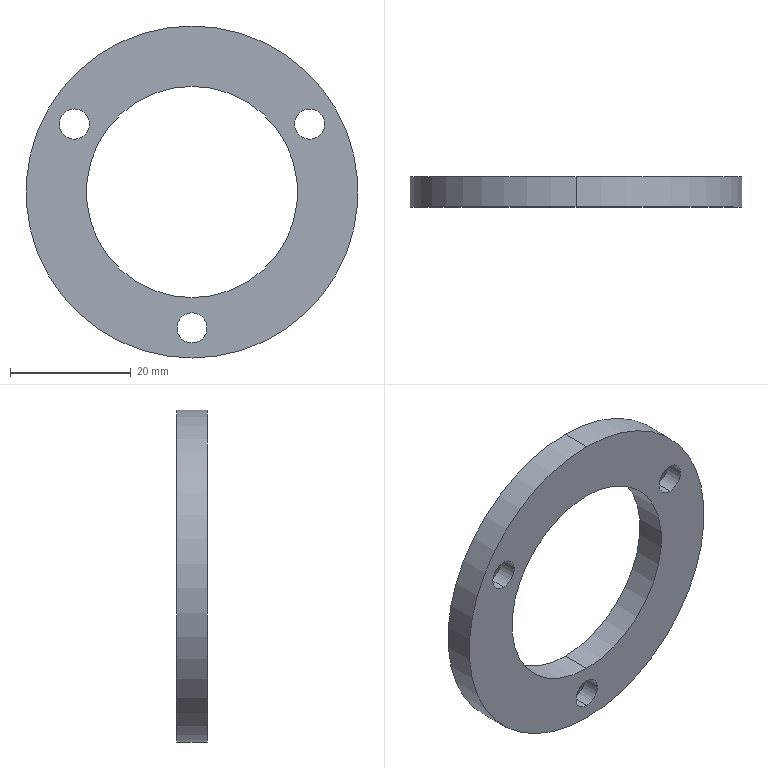Part | SolidWorks | features Extrusion 1, HoleWzd 1 | 1 solid | 18 faces | box 55 x 5 x 55 mm | volume 6655 mm3 | cylinder 10 | cone 6 | plane 2 | commonest cylinder face diameters 5 x6 35 x2 55 x2
STEP:
#1=CARTESIAN_POINT('',(0.,3.,-25.));
#2=VERTEX_POINT('',#1);
#3=CARTESIAN_POINT('',(0.,3.,-20.));
#4=VERTEX_POINT('',#3);
#5=CARTESIAN_POINT('',(0.,3.,-22.5));
#6=DIRECTION('',(0.,1.,0.));
#7=DIRECTION('',(0.,0.,1.));
#8=AXIS2_PLACEMENT_3D('',#5,#6,#7);
#9=CIRCLE('',#8,2.5);
#10=EDGE_CURVE('',#2,#4,#9,.T.);
#11=ORIENTED_EDGE('',*,*,#10,.F.);
#12=CARTESIAN_POINT('',(0.,5.,-27.));
#13=VERTEX_POINT('',#12);
#14=CARTESIAN_POINT('',(0.,5.,-27.));
#15=DIRECTION('',(0.,0.7071,-0.7071));
#16=VECTOR('',#15,1000.);
#17=LINE('',#14,#16);
#18=EDGE_CURVE('',#2,#13,#17,.T.);
#19=ORIENTED_EDGE('',*,*,#18,.T.);
#20=CARTESIAN_POINT('',(0.,5.,-18.));
#21=VERTEX_POINT('',#20);
#22=CARTESIAN_POINT('',(0.,5.,-22.5));
#23=DIRECTION('',(0.,1.,0.));
#24=DIRECTION('',(0.,0.,1.));
#25=AXIS2_PLACEMENT_3D('',#22,#23,#24);
#26=CIRCLE('',#25,4.5);
#27=EDGE_CURVE('',#13,#21,#26,.T.);
#28=ORIENTED_EDGE('',*,*,#27,.T.);
#29=CARTESIAN_POINT('',(0.,5.,-18.));
#30=DIRECTION('',(0.,0.7071,0.7071));
#31=VECTOR('',#30,1000.);
#32=LINE('',#29,#31);
#33=EDGE_CURVE('',#4,#21,#32,.T.);
#34=ORIENTED_EDGE('',*,*,#33,.F.);
#35=EDGE_LOOP('',(#11,#19,#28,#34));
#36=FACE_OUTER_BOUND('',#35,.T.);
#37=CARTESIAN_POINT('',(0.,5.,-22.5));
#38=DIRECTION('',(0.,1.,0.));
#39=DIRECTION('',(0.,0.,1.));
#40=AXIS2_PLACEMENT_3D('',#37,#38,#39);
#41=CONICAL_SURFACE('',#40,4.5,0.7854);
#42=ADVANCED_FACE('',(#36),#41,.F.);
#43=CARTESIAN_POINT('',(0.,0.,-25.));
#44=VERTEX_POINT('',#43);
#45=CARTESIAN_POINT('',(0.,0.,-20.));
#46=VERTEX_POINT('',#45);
#47=CARTESIAN_POINT('',(0.,0.,-22.5));
#48=DIRECTION('',(0.,1.,0.));
#49=DIRECTION('',(0.,0.,1.));
#50=AXIS2_PLACEMENT_3D('',#47,#48,#49);
#51=CIRCLE('',#50,2.5);
#52=EDGE_CURVE('',#44,#46,#51,.T.);
#53=ORIENTED_EDGE('',*,*,#52,.F.);
#54=CARTESIAN_POINT('',(0.,5.,-25.));
#55=DIRECTION('',(0.,1.,0.));
#56=VECTOR('',#55,1000.);
#57=LINE('',#54,#56);
#58=EDGE_CURVE('',#44,#2,#57,.T.);
#59=ORIENTED_EDGE('',*,*,#58,.T.);
#60=ORIENTED_EDGE('',*,*,#10,.T.);
#61=CARTESIAN_POINT('',(0.,5.,-20.));
#62=DIRECTION('',(0.,1.,0.));
#63=VECTOR('',#62,1000.);
#64=LINE('',#61,#63);
#65=EDGE_CURVE('',#46,#4,#64,.T.);
#66=ORIENTED_EDGE('',*,*,#65,.F.);
#67=EDGE_LOOP('',(#53,#59,#60,#66));
#68=FACE_OUTER_BOUND('',#67,.T.);
#69=CARTESIAN_POINT('',(0.,5.,-22.5));
#70=DIRECTION('',(0.,1.,0.));
#71=DIRECTION('',(0.,0.,1.));
#72=AXIS2_PLACEMENT_3D('',#69,#70,#71);
#73=CYLINDRICAL_SURFACE('',#72,2.5);
#74=ADVANCED_FACE('',(#68),#73,.F.);
#75=CARTESIAN_POINT('',(19.486,3.,8.75));
#76=VERTEX_POINT('',#75);
#77=CARTESIAN_POINT('',(19.486,3.,13.75));
#78=VERTEX_POINT('',#77);
#79=CARTESIAN_POINT('',(19.486,3.,11.25));
#80=DIRECTION('',(0.,1.,0.));
#81=DIRECTION('',(0.,0.,1.));
#82=AXIS2_PLACEMENT_3D('',#79,#80,#81);
#83=CIRCLE('',#82,2.5);
#84=EDGE_CURVE('',#76,#78,#83,.T.);
#85=ORIENTED_EDGE('',*,*,#84,.F.);
#86=CARTESIAN_POINT('',(19.486,5.,6.75));
#87=VERTEX_POINT('',#86);
#88=CARTESIAN_POINT('',(19.486,5.,6.75));
#89=DIRECTION('',(0.,0.7071,-0.7071));
#90=VECTOR('',#89,1000.);
#91=LINE('',#88,#90);
#92=EDGE_CURVE('',#76,#87,#91,.T.);
#93=ORIENTED_EDGE('',*,*,#92,.T.);
#94=CARTESIAN_POINT('',(19.486,5.,15.75));
#95=VERTEX_POINT('',#94);
#96=CARTESIAN_POINT('',(19.486,5.,11.25));
#97=DIRECTION('',(0.,1.,0.));
#98=DIRECTION('',(0.,0.,1.));
#99=AXIS2_PLACEMENT_3D('',#96,#97,#98);
#100=CIRCLE('',#99,4.5);
#101=EDGE_CURVE('',#87,#95,#100,.T.);
#102=ORIENTED_EDGE('',*,*,#101,.T.);
#103=CARTESIAN_POINT('',(19.486,5.,15.75));
#104=DIRECTION('',(0.,0.7071,0.7071));
#105=VECTOR('',#104,1000.);
#106=LINE('',#103,#105);
#107=EDGE_CURVE('',#78,#95,#106,.T.);
#108=ORIENTED_EDGE('',*,*,#107,.F.);
#109=EDGE_LOOP('',(#85,#93,#102,#108));
#110=FACE_OUTER_BOUND('',#109,.T.);
#111=CARTESIAN_POINT('',(19.486,5.,11.25));
#112=DIRECTION('',(0.,1.,0.));
#113=DIRECTION('',(0.,0.,1.));
#114=AXIS2_PLACEMENT_3D('',#111,#112,#113);
#115=CONICAL_SURFACE('',#114,4.5,0.7854);
#116=ADVANCED_FACE('',(#110),#115,.F.);
#117=CARTESIAN_POINT('',(19.486,0.,8.75));
#118=VERTEX_POINT('',#117);
#119=CARTESIAN_POINT('',(19.486,0.,13.75));
#120=VERTEX_POINT('',#119);
#121=CARTESIAN_POINT('',(19.486,0.,11.25));
#122=DIRECTION('',(0.,1.,0.));
#123=DIRECTION('',(0.,0.,1.));
#124=AXIS2_PLACEMENT_3D('',#121,#122,#123);
#125=CIRCLE('',#124,2.5);
#126=EDGE_CURVE('',#118,#120,#125,.T.);
#127=ORIENTED_EDGE('',*,*,#126,.F.);
#128=CARTESIAN_POINT('',(19.486,5.,8.75));
#129=DIRECTION('',(0.,1.,0.));
#130=VECTOR('',#129,1000.);
#131=LINE('',#128,#130);
#132=EDGE_CURVE('',#118,#76,#131,.T.);
#133=ORIENTED_EDGE('',*,*,#132,.T.);
#134=ORIENTED_EDGE('',*,*,#84,.T.);
#135=CARTESIAN_POINT('',(19.486,5.,13.75));
#136=DIRECTION('',(0.,1.,0.));
#137=VECTOR('',#136,1000.);
#138=LINE('',#135,#137);
#139=EDGE_CURVE('',#120,#78,#138,.T.);
#140=ORIENTED_EDGE('',*,*,#139,.F.);
#141=EDGE_LOOP('',(#127,#133,#134,#140));
#142=FACE_OUTER_BOUND('',#141,.T.);
#143=CARTESIAN_POINT('',(19.486,5.,11.25));
#144=DIRECTION('',(0.,1.,0.));
#145=DIRECTION('',(0.,0.,1.));
#146=AXIS2_PLACEMENT_3D('',#143,#144,#145);
#147=CYLINDRICAL_SURFACE('',#146,2.5);
#148=ADVANCED_FACE('',(#142),#147,.F.);
#149=CARTESIAN_POINT('',(-19.486,3.,8.75));
#150=VERTEX_POINT('',#149);
#151=CARTESIAN_POINT('',(-19.486,3.,13.75));
#152=VERTEX_POINT('',#151);
#153=CARTESIAN_POINT('',(-19.486,3.,11.25));
#154=DIRECTION('',(0.,1.,0.));
#155=DIRECTION('',(0.,0.,1.));
#156=AXIS2_PLACEMENT_3D('',#153,#154,#155);
#157=CIRCLE('',#156,2.5);
#158=EDGE_CURVE('',#150,#152,#157,.T.);
#159=ORIENTED_EDGE('',*,*,#158,.F.);
#160=CARTESIAN_POINT('',(-19.486,5.,6.75));
#161=VERTEX_POINT('',#160);
#162=CARTESIAN_POINT('',(-19.486,5.,6.75));
#163=DIRECTION('',(0.,0.7071,-0.7071));
#164=VECTOR('',#163,1000.);
#165=LINE('',#162,#164);
#166=EDGE_CURVE('',#150,#161,#165,.T.);
#167=ORIENTED_EDGE('',*,*,#166,.T.);
#168=CARTESIAN_POINT('',(-19.486,5.,15.75));
#169=VERTEX_POINT('',#168);
#170=CARTESIAN_POINT('',(-19.486,5.,11.25));
#171=DIRECTION('',(0.,1.,0.));
#172=DIRECTION('',(0.,0.,1.));
#173=AXIS2_PLACEMENT_3D('',#170,#171,#172);
#174=CIRCLE('',#173,4.5);
#175=EDGE_CURVE('',#161,#169,#174,.T.);
#176=ORIENTED_EDGE('',*,*,#175,.T.);
#177=CARTESIAN_POINT('',(-19.486,5.,15.75));
#178=DIRECTION('',(0.,0.7071,0.7071));
#179=VECTOR('',#178,1000.);
#180=LINE('',#177,#179);
#181=EDGE_CURVE('',#152,#169,#180,.T.);
#182=ORIENTED_EDGE('',*,*,#181,.F.);
#183=EDGE_LOOP('',(#159,#167,#176,#182));
#184=FACE_OUTER_BOUND('',#183,.T.);
#185=CARTESIAN_POINT('',(-19.486,5.,11.25));
#186=DIRECTION('',(0.,1.,0.));
#187=DIRECTION('',(0.,0.,1.));
#188=AXIS2_PLACEMENT_3D('',#185,#186,#187);
#189=CONICAL_SURFACE('',#188,4.5,0.7854);
#190=ADVANCED_FACE('',(#184),#189,.F.);
#191=CARTESIAN_POINT('',(-19.486,0.,8.75));
#192=VERTEX_POINT('',#191);
#193=CARTESIAN_POINT('',(-19.486,0.,13.75));
#194=VERTEX_POINT('',#193);
#195=CARTESIAN_POINT('',(-19.486,0.,11.25));
#196=DIRECTION('',(0.,1.,0.));
#197=DIRECTION('',(0.,0.,1.));
#198=AXIS2_PLACEMENT_3D('',#195,#196,#197);
#199=CIRCLE('',#198,2.5);
#200=EDGE_CURVE('',#192,#194,#199,.T.);
#201=ORIENTED_EDGE('',*,*,#200,.F.);
#202=CARTESIAN_POINT('',(-19.486,5.,8.75));
#203=DIRECTION('',(0.,1.,0.));
#204=VECTOR('',#203,1000.);
#205=LINE('',#202,#204);
#206=EDGE_CURVE('',#192,#150,#205,.T.);
#207=ORIENTED_EDGE('',*,*,#206,.T.);
#208=ORIENTED_EDGE('',*,*,#158,.T.);
#209=CARTESIAN_POINT('',(-19.486,5.,13.75));
#210=DIRECTION('',(0.,1.,0.));
#211=VECTOR('',#210,1000.);
#212=LINE('',#209,#211);
#213=EDGE_CURVE('',#194,#152,#212,.T.);
#214=ORIENTED_EDGE('',*,*,#213,.F.);
#215=EDGE_LOOP('',(#201,#207,#208,#214));
#216=FACE_OUTER_BOUND('',#215,.T.);
#217=CARTESIAN_POINT('',(-19.486,5.,11.25));
#218=DIRECTION('',(0.,1.,0.));
#219=DIRECTION('',(0.,0.,1.));
#220=AXIS2_PLACEMENT_3D('',#217,#218,#219);
#221=CYLINDRICAL_SURFACE('',#220,2.5);
#222=ADVANCED_FACE('',(#216),#221,.F.);
#223=CARTESIAN_POINT('',(0.,5.,-17.5));
#224=VERTEX_POINT('',#223);
#225=CARTESIAN_POINT('',(0.,5.,17.5));
#226=VERTEX_POINT('',#225);
#227=CARTESIAN_POINT('',(0.,5.,0.));
#228=DIRECTION('',(0.,1.,0.));
#229=DIRECTION('',(0.,0.,1.));
#230=AXIS2_PLACEMENT_3D('',#227,#228,#229);
#231=CIRCLE('',#230,17.5);
#232=EDGE_CURVE('',#224,#226,#231,.T.);
#233=ORIENTED_EDGE('',*,*,#232,.T.);
#234=CARTESIAN_POINT('',(0.,0.,17.5));
#235=VERTEX_POINT('',#234);
#236=CARTESIAN_POINT('',(0.,5.,17.5));
#237=DIRECTION('',(0.,-1.,0.));
#238=VECTOR('',#237,1000.);
#239=LINE('',#236,#238);
#240=EDGE_CURVE('',#226,#235,#239,.T.);
#241=ORIENTED_EDGE('',*,*,#240,.T.);
#242=CARTESIAN_POINT('',(0.,0.,-17.5));
#243=VERTEX_POINT('',#242);
#244=CARTESIAN_POINT('',(0.,0.,0.));
#245=DIRECTION('',(0.,1.,0.));
#246=DIRECTION('',(0.,0.,1.));
#247=AXIS2_PLACEMENT_3D('',#244,#245,#246);
#248=CIRCLE('',#247,17.5);
#249=EDGE_CURVE('',#243,#235,#248,.T.);
#250=ORIENTED_EDGE('',*,*,#249,.F.);
#251=CARTESIAN_POINT('',(0.,5.,-17.5));
#252=DIRECTION('',(0.,-1.,0.));
#253=VECTOR('',#252,1000.);
#254=LINE('',#251,#253);
#255=EDGE_CURVE('',#224,#243,#254,.T.);
#256=ORIENTED_EDGE('',*,*,#255,.F.);
#257=EDGE_LOOP('',(#233,#241,#250,#256));
#258=FACE_OUTER_BOUND('',#257,.T.);
#259=CARTESIAN_POINT('',(0.,5.,0.));
#260=DIRECTION('',(0.,-1.,0.));
#261=DIRECTION('',(0.,0.,-1.));
#262=AXIS2_PLACEMENT_3D('',#259,#260,#261);
#263=CYLINDRICAL_SURFACE('',#262,17.5);
#264=ADVANCED_FACE('',(#258),#263,.F.);
#265=CARTESIAN_POINT('',(0.,5.,27.5));
#266=VERTEX_POINT('',#265);
#267=CARTESIAN_POINT('',(0.,5.,-27.5));
#268=VERTEX_POINT('',#267);
#269=CARTESIAN_POINT('',(0.,5.,0.));
#270=DIRECTION('',(0.,1.,0.));
#271=DIRECTION('',(0.,0.,1.));
#272=AXIS2_PLACEMENT_3D('',#269,#270,#271);
#273=CIRCLE('',#272,27.5);
#274=EDGE_CURVE('',#266,#268,#273,.T.);
#275=ORIENTED_EDGE('',*,*,#274,.F.);
#276=CARTESIAN_POINT('',(0.,0.,27.5));
#277=VERTEX_POINT('',#276);
#278=CARTESIAN_POINT('',(0.,5.,27.5));
#279=DIRECTION('',(0.,-1.,0.));
#280=VECTOR('',#279,1000.);
#281=LINE('',#278,#280);
#282=EDGE_CURVE('',#266,#277,#281,.T.);
#283=ORIENTED_EDGE('',*,*,#282,.T.);
#284=CARTESIAN_POINT('',(0.,0.,-27.5));
#285=VERTEX_POINT('',#284);
#286=CARTESIAN_POINT('',(0.,0.,0.));
#287=DIRECTION('',(0.,1.,0.));
#288=DIRECTION('',(0.,0.,1.));
#289=AXIS2_PLACEMENT_3D('',#286,#287,#288);
#290=CIRCLE('',#289,27.5);
#291=EDGE_CURVE('',#277,#285,#290,.T.);
#292=ORIENTED_EDGE('',*,*,#291,.T.);
#293=CARTESIAN_POINT('',(0.,5.,-27.5));
#294=DIRECTION('',(0.,-1.,0.));
#295=VECTOR('',#294,1000.);
#296=LINE('',#293,#295);
#297=EDGE_CURVE('',#268,#285,#296,.T.);
#298=ORIENTED_EDGE('',*,*,#297,.F.);
#299=EDGE_LOOP('',(#275,#283,#292,#298));
#300=FACE_OUTER_BOUND('',#299,.T.);
#301=CARTESIAN_POINT('',(0.,5.,0.));
#302=DIRECTION('',(0.,-1.,0.));
#303=DIRECTION('',(0.,0.,-1.));
#304=AXIS2_PLACEMENT_3D('',#301,#302,#303);
#305=CYLINDRICAL_SURFACE('',#304,27.5);
#306=ADVANCED_FACE('',(#300),#305,.T.);
#307=CARTESIAN_POINT('',(0.,5.,-22.5));
#308=DIRECTION('',(0.,1.,0.));
#309=DIRECTION('',(0.,0.,1.));
#310=AXIS2_PLACEMENT_3D('',#307,#308,#309);
#311=CIRCLE('',#310,4.5);
#312=EDGE_CURVE('',#21,#13,#311,.T.);
#313=ORIENTED_EDGE('',*,*,#312,.F.);
#314=ORIENTED_EDGE('',*,*,#27,.F.);
#315=EDGE_LOOP('',(#313,#314));
#316=FACE_BOUND('',#315,.T.);
#317=CARTESIAN_POINT('',(19.486,5.,11.25));
#318=DIRECTION('',(0.,1.,0.));
#319=DIRECTION('',(0.,0.,1.));
#320=AXIS2_PLACEMENT_3D('',#317,#318,#319);
#321=CIRCLE('',#320,4.5);
#322=EDGE_CURVE('',#95,#87,#321,.T.);
#323=ORIENTED_EDGE('',*,*,#322,.F.);
#324=ORIENTED_EDGE('',*,*,#101,.F.);
#325=EDGE_LOOP('',(#323,#324));
#326=FACE_BOUND('',#325,.T.);
#327=CARTESIAN_POINT('',(-19.486,5.,11.25));
#328=DIRECTION('',(0.,1.,0.));
#329=DIRECTION('',(0.,0.,1.));
#330=AXIS2_PLACEMENT_3D('',#327,#328,#329);
#331=CIRCLE('',#330,4.5);
#332=EDGE_CURVE('',#169,#161,#331,.T.);
#333=ORIENTED_EDGE('',*,*,#332,.F.);
#334=ORIENTED_EDGE('',*,*,#175,.F.);
#335=EDGE_LOOP('',(#333,#334));
#336=FACE_BOUND('',#335,.T.);
#337=CARTESIAN_POINT('',(0.,5.,0.));
#338=DIRECTION('',(0.,1.,0.));
#339=DIRECTION('',(0.,0.,1.));
#340=AXIS2_PLACEMENT_3D('',#337,#338,#339);
#341=CIRCLE('',#340,27.5);
#342=EDGE_CURVE('',#268,#266,#341,.T.);
#343=ORIENTED_EDGE('',*,*,#342,.T.);
#344=ORIENTED_EDGE('',*,*,#274,.T.);
#345=EDGE_LOOP('',(#343,#344));
#346=FACE_OUTER_BOUND('',#345,.T.);
#347=ORIENTED_EDGE('',*,*,#232,.F.);
#348=CARTESIAN_POINT('',(0.,5.,0.));
#349=DIRECTION('',(0.,1.,0.));
#350=DIRECTION('',(0.,0.,1.));
#351=AXIS2_PLACEMENT_3D('',#348,#349,#350);
#352=CIRCLE('',#351,17.5);
#353=EDGE_CURVE('',#226,#224,#352,.T.);
#354=ORIENTED_EDGE('',*,*,#353,.F.);
#355=EDGE_LOOP('',(#347,#354));
#356=FACE_BOUND('',#355,.T.);
#357=CARTESIAN_POINT('',(0.,5.,0.));
#358=DIRECTION('',(0.,1.,0.));
#359=DIRECTION('',(0.,0.,1.));
#360=AXIS2_PLACEMENT_3D('',#357,#358,#359);
#361=PLANE('',#360);
#362=ADVANCED_FACE('',(#316,#326,#336,#346,#356),#361,.T.);
#363=CARTESIAN_POINT('',(0.,0.,-22.5));
#364=DIRECTION('',(0.,1.,0.));
#365=DIRECTION('',(0.,0.,1.));
#366=AXIS2_PLACEMENT_3D('',#363,#364,#365);
#367=CIRCLE('',#366,2.5);
#368=EDGE_CURVE('',#46,#44,#367,.T.);
#369=ORIENTED_EDGE('',*,*,#368,.T.);
#370=ORIENTED_EDGE('',*,*,#52,.T.);
#371=EDGE_LOOP('',(#369,#370));
#372=FACE_BOUND('',#371,.T.);
#373=CARTESIAN_POINT('',(19.486,0.,11.25));
#374=DIRECTION('',(0.,1.,0.));
#375=DIRECTION('',(0.,0.,1.));
#376=AXIS2_PLACEMENT_3D('',#373,#374,#375);
#377=CIRCLE('',#376,2.5);
#378=EDGE_CURVE('',#120,#118,#377,.T.);
#379=ORIENTED_EDGE('',*,*,#378,.T.);
#380=ORIENTED_EDGE('',*,*,#126,.T.);
#381=EDGE_LOOP('',(#379,#380));
#382=FACE_BOUND('',#381,.T.);
#383=CARTESIAN_POINT('',(-19.486,0.,11.25));
#384=DIRECTION('',(0.,1.,0.));
#385=DIRECTION('',(0.,0.,1.));
#386=AXIS2_PLACEMENT_3D('',#383,#384,#385);
#387=CIRCLE('',#386,2.5);
#388=EDGE_CURVE('',#194,#192,#387,.T.);
#389=ORIENTED_EDGE('',*,*,#388,.T.);
#390=ORIENTED_EDGE('',*,*,#200,.T.);
#391=EDGE_LOOP('',(#389,#390));
#392=FACE_BOUND('',#391,.T.);
#393=CARTESIAN_POINT('',(0.,0.,0.));
#394=DIRECTION('',(0.,1.,0.));
#395=DIRECTION('',(0.,0.,1.));
#396=AXIS2_PLACEMENT_3D('',#393,#394,#395);
#397=CIRCLE('',#396,27.5);
#398=EDGE_CURVE('',#285,#277,#397,.T.);
#399=ORIENTED_EDGE('',*,*,#398,.F.);
#400=ORIENTED_EDGE('',*,*,#291,.F.);
#401=EDGE_LOOP('',(#399,#400));
#402=FACE_OUTER_BOUND('',#401,.T.);
#403=ORIENTED_EDGE('',*,*,#249,.T.);
#404=CARTESIAN_POINT('',(0.,0.,0.));
#405=DIRECTION('',(0.,1.,0.));
#406=DIRECTION('',(0.,0.,1.));
#407=AXIS2_PLACEMENT_3D('',#404,#405,#406);
#408=CIRCLE('',#407,17.5);
#409=EDGE_CURVE('',#235,#243,#408,.T.);
#410=ORIENTED_EDGE('',*,*,#409,.T.);
#411=EDGE_LOOP('',(#403,#410));
#412=FACE_BOUND('',#411,.T.);
#413=CARTESIAN_POINT('',(0.,0.,0.));
#414=DIRECTION('',(0.,1.,0.));
#415=DIRECTION('',(0.,0.,1.));
#416=AXIS2_PLACEMENT_3D('',#413,#414,#415);
#417=PLANE('',#416);
#418=ADVANCED_FACE('',(#372,#382,#392,#402,#412),#417,.F.);
#419=ORIENTED_EDGE('',*,*,#282,.F.);
#420=ORIENTED_EDGE('',*,*,#342,.F.);
#421=ORIENTED_EDGE('',*,*,#297,.T.);
#422=ORIENTED_EDGE('',*,*,#398,.T.);
#423=EDGE_LOOP('',(#419,#420,#421,#422));
#424=FACE_OUTER_BOUND('',#423,.T.);
#425=CARTESIAN_POINT('',(0.,5.,0.));
#426=DIRECTION('',(0.,-1.,0.));
#427=DIRECTION('',(0.,0.,-1.));
#428=AXIS2_PLACEMENT_3D('',#425,#426,#427);
#429=CYLINDRICAL_SURFACE('',#428,27.5);
#430=ADVANCED_FACE('',(#424),#429,.T.);
#431=ORIENTED_EDGE('',*,*,#240,.F.);
#432=ORIENTED_EDGE('',*,*,#353,.T.);
#433=ORIENTED_EDGE('',*,*,#255,.T.);
#434=ORIENTED_EDGE('',*,*,#409,.F.);
#435=EDGE_LOOP('',(#431,#432,#433,#434));
#436=FACE_OUTER_BOUND('',#435,.T.);
#437=CARTESIAN_POINT('',(0.,5.,0.));
#438=DIRECTION('',(0.,-1.,0.));
#439=DIRECTION('',(0.,0.,-1.));
#440=AXIS2_PLACEMENT_3D('',#437,#438,#439);
#441=CYLINDRICAL_SURFACE('',#440,17.5);
#442=ADVANCED_FACE('',(#436),#441,.F.);
#443=ORIENTED_EDGE('',*,*,#206,.F.);
#444=ORIENTED_EDGE('',*,*,#388,.F.);
#445=ORIENTED_EDGE('',*,*,#213,.T.);
#446=CARTESIAN_POINT('',(-19.486,3.,11.25));
#447=DIRECTION('',(0.,1.,0.));
#448=DIRECTION('',(0.,0.,1.));
#449=AXIS2_PLACEMENT_3D('',#446,#447,#448);
#450=CIRCLE('',#449,2.5);
#451=EDGE_CURVE('',#152,#150,#450,.T.);
#452=ORIENTED_EDGE('',*,*,#451,.T.);
#453=EDGE_LOOP('',(#443,#444,#445,#452));
#454=FACE_OUTER_BOUND('',#453,.T.);
#455=CARTESIAN_POINT('',(-19.486,5.,11.25));
#456=DIRECTION('',(0.,1.,0.));
#457=DIRECTION('',(0.,0.,1.));
#458=AXIS2_PLACEMENT_3D('',#455,#456,#457);
#459=CYLINDRICAL_SURFACE('',#458,2.5);
#460=ADVANCED_FACE('',(#454),#459,.F.);
#461=ORIENTED_EDGE('',*,*,#166,.F.);
#462=ORIENTED_EDGE('',*,*,#451,.F.);
#463=ORIENTED_EDGE('',*,*,#181,.T.);
#464=ORIENTED_EDGE('',*,*,#332,.T.);
#465=EDGE_LOOP('',(#461,#462,#463,#464));
#466=FACE_OUTER_BOUND('',#465,.T.);
#467=CARTESIAN_POINT('',(-19.486,5.,11.25));
#468=DIRECTION('',(0.,1.,0.));
#469=DIRECTION('',(0.,0.,1.));
#470=AXIS2_PLACEMENT_3D('',#467,#468,#469);
#471=CONICAL_SURFACE('',#470,4.5,0.7854);
#472=ADVANCED_FACE('',(#466),#471,.F.);
#473=ORIENTED_EDGE('',*,*,#132,.F.);
#474=ORIENTED_EDGE('',*,*,#378,.F.);
#475=ORIENTED_EDGE('',*,*,#139,.T.);
#476=CARTESIAN_POINT('',(19.486,3.,11.25));
#477=DIRECTION('',(0.,1.,0.));
#478=DIRECTION('',(0.,0.,1.));
#479=AXIS2_PLACEMENT_3D('',#476,#477,#478);
#480=CIRCLE('',#479,2.5);
#481=EDGE_CURVE('',#78,#76,#480,.T.);
#482=ORIENTED_EDGE('',*,*,#481,.T.);
#483=EDGE_LOOP('',(#473,#474,#475,#482));
#484=FACE_OUTER_BOUND('',#483,.T.);
#485=CARTESIAN_POINT('',(19.486,5.,11.25));
#486=DIRECTION('',(0.,1.,0.));
#487=DIRECTION('',(0.,0.,1.));
#488=AXIS2_PLACEMENT_3D('',#485,#486,#487);
#489=CYLINDRICAL_SURFACE('',#488,2.5);
#490=ADVANCED_FACE('',(#484),#489,.F.);
#491=ORIENTED_EDGE('',*,*,#92,.F.);
#492=ORIENTED_EDGE('',*,*,#481,.F.);
#493=ORIENTED_EDGE('',*,*,#107,.T.);
#494=ORIENTED_EDGE('',*,*,#322,.T.);
#495=EDGE_LOOP('',(#491,#492,#493,#494));
#496=FACE_OUTER_BOUND('',#495,.T.);
#497=CARTESIAN_POINT('',(19.486,5.,11.25));
#498=DIRECTION('',(0.,1.,0.));
#499=DIRECTION('',(0.,0.,1.));
#500=AXIS2_PLACEMENT_3D('',#497,#498,#499);
#501=CONICAL_SURFACE('',#500,4.5,0.7854);
#502=ADVANCED_FACE('',(#496),#501,.F.);
#503=ORIENTED_EDGE('',*,*,#58,.F.);
#504=ORIENTED_EDGE('',*,*,#368,.F.);
#505=ORIENTED_EDGE('',*,*,#65,.T.);
#506=CARTESIAN_POINT('',(0.,3.,-22.5));
#507=DIRECTION('',(0.,1.,0.));
#508=DIRECTION('',(0.,0.,1.));
#509=AXIS2_PLACEMENT_3D('',#506,#507,#508);
#510=CIRCLE('',#509,2.5);
#511=EDGE_CURVE('',#4,#2,#510,.T.);
#512=ORIENTED_EDGE('',*,*,#511,.T.);
#513=EDGE_LOOP('',(#503,#504,#505,#512));
#514=FACE_OUTER_BOUND('',#513,.T.);
#515=CARTESIAN_POINT('',(0.,5.,-22.5));
#516=DIRECTION('',(0.,1.,0.));
#517=DIRECTION('',(0.,0.,1.));
#518=AXIS2_PLACEMENT_3D('',#515,#516,#517);
#519=CYLINDRICAL_SURFACE('',#518,2.5);
#520=ADVANCED_FACE('',(#514),#519,.F.);
#521=ORIENTED_EDGE('',*,*,#18,.F.);
#522=ORIENTED_EDGE('',*,*,#511,.F.);
#523=ORIENTED_EDGE('',*,*,#33,.T.);
#524=ORIENTED_EDGE('',*,*,#312,.T.);
#525=EDGE_LOOP('',(#521,#522,#523,#524));
#526=FACE_OUTER_BOUND('',#525,.T.);
#527=CARTESIAN_POINT('',(0.,5.,-22.5));
#528=DIRECTION('',(0.,1.,0.));
#529=DIRECTION('',(0.,0.,1.));
#530=AXIS2_PLACEMENT_3D('',#527,#528,#529);
#531=CONICAL_SURFACE('',#530,4.5,0.7854);
#532=ADVANCED_FACE('',(#526),#531,.F.);
#533=CLOSED_SHELL('',(#42,#74,#116,#148,#190,#222,#264,#306,#362,#418,#430,#442,#460,#472,#490,#502,#520,#532));
#534=MANIFOLD_SOLID_BREP('',#533);
#535=CARTESIAN_POINT('',(0.,0.,0.));
#536=DIRECTION('',(0.,0.,1.));
#537=DIRECTION('',(1.,0.,0.));
#538=AXIS2_PLACEMENT_3D('',#535,#536,#537);
#539=(LENGTH_UNIT()NAMED_UNIT(*)SI_UNIT(.MILLI.,.METRE.));
#540=UNCERTAINTY_MEASURE_WITH_UNIT(LENGTH_MEASURE(0.00001),#539,'','');
#541=(NAMED_UNIT(*)PLANE_ANGLE_UNIT()SI_UNIT($,.RADIAN.));
#542=(NAMED_UNIT(*)SI_UNIT($,.STERADIAN.)SOLID_ANGLE_UNIT());
#543=(GEOMETRIC_REPRESENTATION_CONTEXT(3)GLOBAL_UNCERTAINTY_ASSIGNED_CONTEXT((#540))GLOBAL_UNIT_ASSIGNED_CONTEXT((#539,#541,#542))REPRESENTATION_CONTEXT('',''));
#544=ADVANCED_BREP_SHAPE_REPRESENTATION('',(#534,#538),#543);